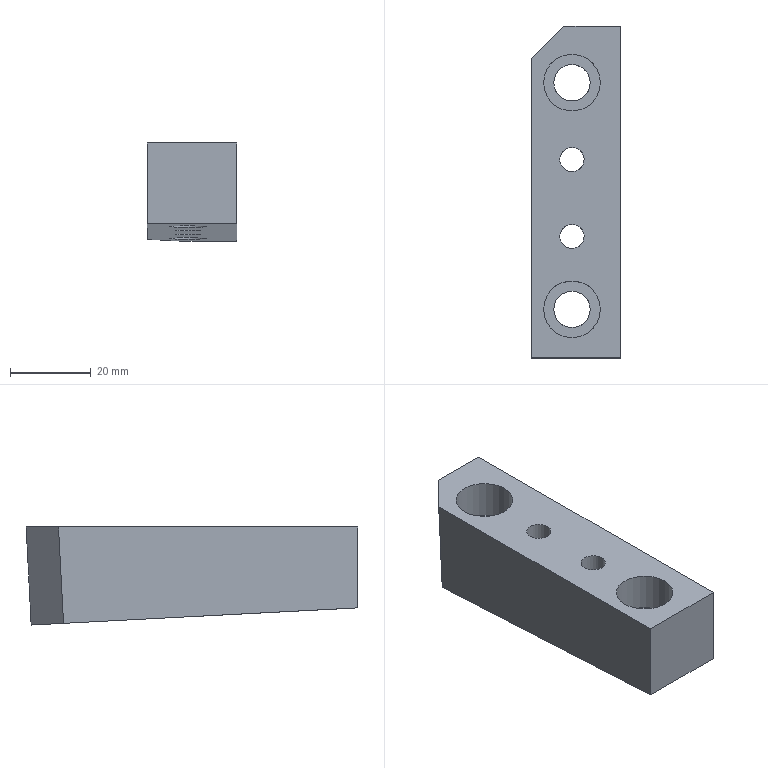Part | STEP file | P011002S001-004 | 1 solid | 15 faces | box 22 x 82 x 24.22 mm | volume 33052 mm3 | plane 9 | cylinder 6 | commonest cylinder face diameters 6 x2 9 x2 14 x2
STEP:
#1=CARTESIAN_POINT('',(0.,0.,0.));
#2=DIRECTION('',(0.,0.,1.));
#3=DIRECTION('',(1.,0.,0.));
#4=AXIS2_PLACEMENT_3D('',#1,#2,#3);
#5=CARTESIAN_POINT('',(-69.5,280.731,-5.22));
#6=VERTEX_POINT('',#5);
#7=CARTESIAN_POINT('',(-55.5,280.731,-5.22));
#8=VERTEX_POINT('',#7);
#9=CARTESIAN_POINT('',(-55.5,280.731,-5.22));
#10=DIRECTION('',(1.,0.,0.));
#11=VECTOR('',#10,1.);
#12=LINE('',#9,#11);
#13=CARTESIAN_POINT('',(-55.5,257.583,-4.007));
#14=DIRECTION('',(0.,-0.05234,-0.9986));
#15=DIRECTION('',(0.,-0.9986,0.05234));
#16=AXIS2_PLACEMENT_3D('',#13,#14,#15);
#17=PLANE('',#16);
#18=CARTESIAN_POINT('',(-23.18,0.));
#19=DIRECTION('',(0.,-1.));
#20=VECTOR('',#19,1.);
#21=LINE('',#18,#20);
#22=(GEOMETRIC_REPRESENTATION_CONTEXT(2)PARAMETRIC_REPRESENTATION_CONTEXT()REPRESENTATION_CONTEXT('',''));
#23=DEFINITIONAL_REPRESENTATION('',(#21),#22);
#24=PCURVE('',#17,#23);
#25=CARTESIAN_POINT('',(76.5,282.,19.));
#26=DIRECTION('',(0.,0.9986,-0.05234));
#27=DIRECTION('',(0.,0.05234,0.9986));
#28=AXIS2_PLACEMENT_3D('',#25,#26,#27);
#29=PLANE('',#28);
#30=CARTESIAN_POINT('',(-24.253,-132.));
#31=DIRECTION('',(0.,1.));
#32=VECTOR('',#31,1.);
#33=LINE('',#30,#32);
#34=(GEOMETRIC_REPRESENTATION_CONTEXT(2)PARAMETRIC_REPRESENTATION_CONTEXT()REPRESENTATION_CONTEXT('',''));
#35=DEFINITIONAL_REPRESENTATION('',(#33),#34);
#36=PCURVE('',#29,#35);
#37=SURFACE_CURVE('',#12,(#24,#36),.PCURVE_S1.);
#38=EDGE_CURVE('',#6,#8,#37,.T.);
#39=ORIENTED_EDGE('',*,*,#38,.T.);
#40=CARTESIAN_POINT('',(-55.5,200.,-0.989));
#41=VERTEX_POINT('',#40);
#42=CARTESIAN_POINT('',(-55.5,257.583,-4.007));
#43=DIRECTION('',(0.,-0.9986,0.05234));
#44=VECTOR('',#43,1.);
#45=LINE('',#42,#44);
#46=CARTESIAN_POINT('',(0.,0.));
#47=DIRECTION('',(1.,0.));
#48=VECTOR('',#47,1.);
#49=LINE('',#46,#48);
#50=(GEOMETRIC_REPRESENTATION_CONTEXT(2)PARAMETRIC_REPRESENTATION_CONTEXT()REPRESENTATION_CONTEXT('',''));
#51=DEFINITIONAL_REPRESENTATION('',(#49),#50);
#52=PCURVE('',#17,#51);
#53=CARTESIAN_POINT('',(-55.5,257.583,-4.007));
#54=DIRECTION('',(1.,0.,0.));
#55=DIRECTION('',(0.,0.,1.));
#56=AXIS2_PLACEMENT_3D('',#53,#54,#55);
#57=PLANE('',#56);
#58=CARTESIAN_POINT('',(0.,0.));
#59=DIRECTION('',(0.05234,0.9986));
#60=VECTOR('',#59,1.);
#61=LINE('',#58,#60);
#62=(GEOMETRIC_REPRESENTATION_CONTEXT(2)PARAMETRIC_REPRESENTATION_CONTEXT()REPRESENTATION_CONTEXT('',''));
#63=DEFINITIONAL_REPRESENTATION('',(#61),#62);
#64=PCURVE('',#57,#63);
#65=SURFACE_CURVE('',#45,(#52,#64),.PCURVE_S1.);
#66=EDGE_CURVE('',#8,#41,#65,.T.);
#67=ORIENTED_EDGE('',*,*,#66,.T.);
#68=CARTESIAN_POINT('',(-77.5,200.,-0.989));
#69=VERTEX_POINT('',#68);
#70=CARTESIAN_POINT('',(165.,200.,-0.989));
#71=DIRECTION('',(-1.,0.,0.));
#72=VECTOR('',#71,1.);
#73=LINE('',#70,#72);
#74=CARTESIAN_POINT('',(57.662,-220.5));
#75=DIRECTION('',(0.,1.));
#76=VECTOR('',#75,1.);
#77=LINE('',#74,#76);
#78=(GEOMETRIC_REPRESENTATION_CONTEXT(2)PARAMETRIC_REPRESENTATION_CONTEXT()REPRESENTATION_CONTEXT('',''));
#79=DEFINITIONAL_REPRESENTATION('',(#77),#78);
#80=PCURVE('',#17,#79);
#81=CARTESIAN_POINT('',(165.,200.,-50.));
#82=DIRECTION('',(0.,-1.,0.));
#83=DIRECTION('',(0.,0.,-1.));
#84=AXIS2_PLACEMENT_3D('',#81,#82,#83);
#85=PLANE('',#84);
#86=CARTESIAN_POINT('',(-49.011,0.));
#87=DIRECTION('',(0.,-1.));
#88=VECTOR('',#87,1.);
#89=LINE('',#86,#88);
#90=(GEOMETRIC_REPRESENTATION_CONTEXT(2)PARAMETRIC_REPRESENTATION_CONTEXT()REPRESENTATION_CONTEXT('',''));
#91=DEFINITIONAL_REPRESENTATION('',(#89),#90);
#92=PCURVE('',#85,#91);
#93=SURFACE_CURVE('',#73,(#80,#92),.PCURVE_S1.);
#94=EDGE_CURVE('',#41,#69,#93,.T.);
#95=ORIENTED_EDGE('',*,*,#94,.T.);
#96=CARTESIAN_POINT('',(-77.5,272.742,-4.801));
#97=VERTEX_POINT('',#96);
#98=CARTESIAN_POINT('',(-77.5,257.583,-4.007));
#99=DIRECTION('',(0.,-0.9986,0.05234));
#100=VECTOR('',#99,1.);
#101=LINE('',#98,#100);
#102=CARTESIAN_POINT('',(0.,22.));
#103=DIRECTION('',(1.,0.));
#104=VECTOR('',#103,1.);
#105=LINE('',#102,#104);
#106=(GEOMETRIC_REPRESENTATION_CONTEXT(2)PARAMETRIC_REPRESENTATION_CONTEXT()REPRESENTATION_CONTEXT('',''));
#107=DEFINITIONAL_REPRESENTATION('',(#105),#106);
#108=PCURVE('',#17,#107);
#109=CARTESIAN_POINT('',(-77.5,257.583,-4.007));
#110=DIRECTION('',(1.,0.,0.));
#111=DIRECTION('',(0.,0.,1.));
#112=AXIS2_PLACEMENT_3D('',#109,#110,#111);
#113=PLANE('',#112);
#114=CARTESIAN_POINT('',(0.,0.));
#115=DIRECTION('',(0.05234,0.9986));
#116=VECTOR('',#115,1.);
#117=LINE('',#114,#116);
#118=(GEOMETRIC_REPRESENTATION_CONTEXT(2)PARAMETRIC_REPRESENTATION_CONTEXT()REPRESENTATION_CONTEXT('',''));
#119=DEFINITIONAL_REPRESENTATION('',(#117),#118);
#120=PCURVE('',#113,#119);
#121=SURFACE_CURVE('',#101,(#108,#120),.PCURVE_S1.);
#122=EDGE_CURVE('',#97,#69,#121,.T.);
#123=ORIENTED_EDGE('',*,*,#122,.F.);
#124=CARTESIAN_POINT('',(-74.09,276.147,-4.98));
#125=DIRECTION('',(-0.7071,-0.7061,0.03701));
#126=VECTOR('',#125,1.);
#127=LINE('',#124,#126);
#128=CARTESIAN_POINT('',(-18.59,18.59));
#129=DIRECTION('',(0.7071,0.7071));
#130=VECTOR('',#129,1.);
#131=LINE('',#128,#130);
#132=(GEOMETRIC_REPRESENTATION_CONTEXT(2)PARAMETRIC_REPRESENTATION_CONTEXT()REPRESENTATION_CONTEXT('',''));
#133=DEFINITIONAL_REPRESENTATION('',(#131),#132);
#134=PCURVE('',#17,#133);
#135=CARTESIAN_POINT('',(-77.5,272.742,-4.801));
#136=DIRECTION('',(-0.7071,0.7061,-0.03701));
#137=DIRECTION('',(0.7066,0.7076,0.));
#138=AXIS2_PLACEMENT_3D('',#135,#136,#137);
#139=PLANE('',#138);
#140=CARTESIAN_POINT('',(4.819,0.1786));
#141=DIRECTION('',(-0.9993,-0.03703));
#142=VECTOR('',#141,1.);
#143=LINE('',#140,#142);
#144=(GEOMETRIC_REPRESENTATION_CONTEXT(2)PARAMETRIC_REPRESENTATION_CONTEXT()REPRESENTATION_CONTEXT('',''));
#145=DEFINITIONAL_REPRESENTATION('',(#143),#144);
#146=PCURVE('',#139,#145);
#147=SURFACE_CURVE('',#127,(#134,#146),.PCURVE_S1.);
#148=EDGE_CURVE('',#6,#97,#147,.T.);
#149=ORIENTED_EDGE('',*,*,#148,.F.);
#150=EDGE_LOOP('',(#39,#67,#95,#123,#149));
#151=FACE_BOUND('',#150,.T.);
#152=CARTESIAN_POINT('',(-67.5,272.5,-4.789));
#153=VERTEX_POINT('',#152);
#154=CARTESIAN_POINT('',(-63.,268.,-4.553));
#155=VERTEX_POINT('',#154);
#156=CARTESIAN_POINT('',(-67.5,268.,-4.553));
#157=DIRECTION('',(0.,-0.05234,-0.9986));
#158=DIRECTION('',(0.,0.9986,-0.05234));
#159=AXIS2_PLACEMENT_3D('',#156,#157,#158);
#160=ELLIPSE('',#159,4.506,4.5);
#161=CARTESIAN_POINT('',(-10.431,12.));
#162=DIRECTION('',(-1.,0.));
#163=AXIS2_PLACEMENT_2D('',#161,#162);
#164=ELLIPSE('',#163,4.506,4.5);
#165=(GEOMETRIC_REPRESENTATION_CONTEXT(2)PARAMETRIC_REPRESENTATION_CONTEXT()REPRESENTATION_CONTEXT('',''));
#166=DEFINITIONAL_REPRESENTATION('',(#164),#165);
#167=PCURVE('',#17,#166);
#168=CARTESIAN_POINT('',(-67.5,268.,19.));
#169=DIRECTION('',(0.,0.,-1.));
#170=DIRECTION('',(1.,0.,0.));
#171=AXIS2_PLACEMENT_3D('',#168,#169,#170);
#172=CYLINDRICAL_SURFACE('',#171,4.5);
#173=CARTESIAN_POINT('',(4.712,23.789));
#174=CARTESIAN_POINT('',(4.808,23.789));
#175=CARTESIAN_POINT('',(4.998,23.782));
#176=CARTESIAN_POINT('',(5.284,23.754));
#177=CARTESIAN_POINT('',(5.569,23.709));
#178=CARTESIAN_POINT('',(5.855,23.652));
#179=CARTESIAN_POINT('',(6.14,23.587));
#180=CARTESIAN_POINT('',(6.426,23.519));
#181=CARTESIAN_POINT('',(6.712,23.453));
#182=CARTESIAN_POINT('',(6.997,23.396));
#183=CARTESIAN_POINT('',(7.283,23.352));
#184=CARTESIAN_POINT('',(7.568,23.323));
#185=CARTESIAN_POINT('',(7.854,23.314));
#186=CARTESIAN_POINT('',(8.14,23.323));
#187=CARTESIAN_POINT('',(8.425,23.352));
#188=CARTESIAN_POINT('',(8.711,23.396));
#189=CARTESIAN_POINT('',(8.996,23.453));
#190=CARTESIAN_POINT('',(9.282,23.519));
#191=CARTESIAN_POINT('',(9.568,23.587));
#192=CARTESIAN_POINT('',(9.853,23.652));
#193=CARTESIAN_POINT('',(10.139,23.709));
#194=CARTESIAN_POINT('',(10.424,23.754));
#195=CARTESIAN_POINT('',(10.71,23.782));
#196=CARTESIAN_POINT('',(10.9,23.789));
#197=CARTESIAN_POINT('',(10.996,23.789));
#198=B_SPLINE_CURVE_WITH_KNOTS('',3,(#173,#174,#175,#176,#177,#178,#179,#180,#181,#182,#183,#184,#185,#186,#187,#188,#189,#190,#191,#192,#193,#194,#195,#196,#197),.UNSPECIFIED.,.F.,.F.,(4,1,1,1,1,1,1,1,1,1,1,1,1,1,1,1,1,1,1,1,1,1,4),(0.,0.2856,0.5712,0.8568,1.142,1.428,1.714,1.999,2.285,2.57,2.856,3.142,3.427,3.713,3.998,4.284,4.57,4.855,5.141,5.426,5.712,5.998,6.283),.QUASI_UNIFORM_KNOTS.);
#199=(GEOMETRIC_REPRESENTATION_CONTEXT(2)PARAMETRIC_REPRESENTATION_CONTEXT()REPRESENTATION_CONTEXT('',''));
#200=DEFINITIONAL_REPRESENTATION('',(#198),#199);
#201=PCURVE('',#172,#200);
#202=SURFACE_CURVE('',#160,(#167,#201),.PCURVE_S1.);
#203=EDGE_CURVE('',#153,#155,#202,.T.);
#204=ORIENTED_EDGE('',*,*,#203,.F.);
#205=CARTESIAN_POINT('',(-67.5,268.,-4.553));
#206=DIRECTION('',(0.,-0.05234,-0.9986));
#207=DIRECTION('',(0.,0.9986,-0.05234));
#208=AXIS2_PLACEMENT_3D('',#205,#206,#207);
#209=ELLIPSE('',#208,4.506,4.5);
#210=CARTESIAN_POINT('',(-10.431,12.));
#211=DIRECTION('',(-1.,0.));
#212=AXIS2_PLACEMENT_2D('',#210,#211);
#213=ELLIPSE('',#212,4.506,4.5);
#214=(GEOMETRIC_REPRESENTATION_CONTEXT(2)PARAMETRIC_REPRESENTATION_CONTEXT()REPRESENTATION_CONTEXT('',''));
#215=DEFINITIONAL_REPRESENTATION('',(#213),#214);
#216=PCURVE('',#17,#215);
#217=CARTESIAN_POINT('',(-1.571,23.789));
#218=CARTESIAN_POINT('',(-1.476,23.789));
#219=CARTESIAN_POINT('',(-1.285,23.782));
#220=CARTESIAN_POINT('',(-0.9996,23.754));
#221=CARTESIAN_POINT('',(-0.714,23.709));
#222=CARTESIAN_POINT('',(-0.4284,23.652));
#223=CARTESIAN_POINT('',(-0.1428,23.587));
#224=CARTESIAN_POINT('',(0.1428,23.519));
#225=CARTESIAN_POINT('',(0.4284,23.453));
#226=CARTESIAN_POINT('',(0.714,23.396));
#227=CARTESIAN_POINT('',(0.9996,23.352));
#228=CARTESIAN_POINT('',(1.285,23.323));
#229=CARTESIAN_POINT('',(1.571,23.314));
#230=CARTESIAN_POINT('',(1.856,23.323));
#231=CARTESIAN_POINT('',(2.142,23.352));
#232=CARTESIAN_POINT('',(2.428,23.396));
#233=CARTESIAN_POINT('',(2.713,23.453));
#234=CARTESIAN_POINT('',(2.999,23.519));
#235=CARTESIAN_POINT('',(3.284,23.587));
#236=CARTESIAN_POINT('',(3.57,23.652));
#237=CARTESIAN_POINT('',(3.856,23.709));
#238=CARTESIAN_POINT('',(4.141,23.754));
#239=CARTESIAN_POINT('',(4.427,23.782));
#240=CARTESIAN_POINT('',(4.617,23.789));
#241=CARTESIAN_POINT('',(4.712,23.789));
#242=B_SPLINE_CURVE_WITH_KNOTS('',3,(#217,#218,#219,#220,#221,#222,#223,#224,#225,#226,#227,#228,#229,#230,#231,#232,#233,#234,#235,#236,#237,#238,#239,#240,#241),.UNSPECIFIED.,.F.,.F.,(4,1,1,1,1,1,1,1,1,1,1,1,1,1,1,1,1,1,1,1,1,1,4),(0.,0.2856,0.5712,0.8568,1.142,1.428,1.714,1.999,2.285,2.57,2.856,3.142,3.427,3.713,3.998,4.284,4.57,4.855,5.141,5.426,5.712,5.998,6.283),.QUASI_UNIFORM_KNOTS.);
#243=(GEOMETRIC_REPRESENTATION_CONTEXT(2)PARAMETRIC_REPRESENTATION_CONTEXT()REPRESENTATION_CONTEXT('',''));
#244=DEFINITIONAL_REPRESENTATION('',(#242),#243);
#245=PCURVE('',#172,#244);
#246=SURFACE_CURVE('',#209,(#216,#245),.PCURVE_S1.);
#247=EDGE_CURVE('',#155,#153,#246,.T.);
#248=ORIENTED_EDGE('',*,*,#247,.F.);
#249=EDGE_LOOP('',(#204,#248));
#250=FACE_BOUND('',#249,.T.);
#251=CARTESIAN_POINT('',(-67.5,252.,-3.714));
#252=VERTEX_POINT('',#251);
#253=CARTESIAN_POINT('',(-67.5,249.,-3.557));
#254=DIRECTION('',(0.,-0.05234,-0.9986));
#255=DIRECTION('',(0.,0.9986,-0.05234));
#256=AXIS2_PLACEMENT_3D('',#253,#254,#255);
#257=ELLIPSE('',#256,3.004,3.);
#258=CARTESIAN_POINT('',(8.595,12.));
#259=DIRECTION('',(-1.,0.));
#260=AXIS2_PLACEMENT_2D('',#258,#259);
#261=ELLIPSE('',#260,3.004,3.);
#262=(GEOMETRIC_REPRESENTATION_CONTEXT(2)PARAMETRIC_REPRESENTATION_CONTEXT()REPRESENTATION_CONTEXT('',''));
#263=DEFINITIONAL_REPRESENTATION('',(#261),#262);
#264=PCURVE('',#17,#263);
#265=CARTESIAN_POINT('',(-67.5,249.,19.));
#266=DIRECTION('',(0.,0.,-1.));
#267=DIRECTION('',(1.,0.,0.));
#268=AXIS2_PLACEMENT_3D('',#265,#266,#267);
#269=CYLINDRICAL_SURFACE('',#268,3.);
#270=CARTESIAN_POINT('',(4.712,22.714));
#271=CARTESIAN_POINT('',(4.808,22.714));
#272=CARTESIAN_POINT('',(4.998,22.71));
#273=CARTESIAN_POINT('',(5.284,22.691));
#274=CARTESIAN_POINT('',(5.569,22.661));
#275=CARTESIAN_POINT('',(5.855,22.623));
#276=CARTESIAN_POINT('',(6.14,22.58));
#277=CARTESIAN_POINT('',(6.426,22.534));
#278=CARTESIAN_POINT('',(6.712,22.491));
#279=CARTESIAN_POINT('',(6.997,22.453));
#280=CARTESIAN_POINT('',(7.283,22.423));
#281=CARTESIAN_POINT('',(7.568,22.404));
#282=CARTESIAN_POINT('',(7.854,22.398));
#283=CARTESIAN_POINT('',(8.14,22.404));
#284=CARTESIAN_POINT('',(8.425,22.423));
#285=CARTESIAN_POINT('',(8.711,22.453));
#286=CARTESIAN_POINT('',(8.996,22.491));
#287=CARTESIAN_POINT('',(9.282,22.534));
#288=CARTESIAN_POINT('',(9.568,22.58));
#289=CARTESIAN_POINT('',(9.853,22.623));
#290=CARTESIAN_POINT('',(10.139,22.661));
#291=CARTESIAN_POINT('',(10.424,22.691));
#292=CARTESIAN_POINT('',(10.71,22.71));
#293=CARTESIAN_POINT('',(10.9,22.714));
#294=CARTESIAN_POINT('',(10.996,22.714));
#295=B_SPLINE_CURVE_WITH_KNOTS('',3,(#270,#271,#272,#273,#274,#275,#276,#277,#278,#279,#280,#281,#282,#283,#284,#285,#286,#287,#288,#289,#290,#291,#292,#293,#294),.UNSPECIFIED.,.F.,.F.,(4,1,1,1,1,1,1,1,1,1,1,1,1,1,1,1,1,1,1,1,1,1,4),(0.,0.2856,0.5712,0.8568,1.142,1.428,1.714,1.999,2.285,2.57,2.856,3.142,3.427,3.713,3.998,4.284,4.57,4.855,5.141,5.426,5.712,5.998,6.283),.QUASI_UNIFORM_KNOTS.);
#296=(GEOMETRIC_REPRESENTATION_CONTEXT(2)PARAMETRIC_REPRESENTATION_CONTEXT()REPRESENTATION_CONTEXT('',''));
#297=DEFINITIONAL_REPRESENTATION('',(#295),#296);
#298=PCURVE('',#269,#297);
#299=SURFACE_CURVE('',#257,(#264,#298),.PCURVE_S1.);
#300=EDGE_CURVE('',#252,#252,#299,.T.);
#301=ORIENTED_EDGE('',*,*,#300,.F.);
#302=EDGE_LOOP('',(#301));
#303=FACE_BOUND('',#302,.T.);
#304=CARTESIAN_POINT('',(-67.5,233.,-2.718));
#305=VERTEX_POINT('',#304);
#306=CARTESIAN_POINT('',(-67.5,230.,-2.561));
#307=DIRECTION('',(0.,-0.05234,-0.9986));
#308=DIRECTION('',(0.,0.9986,-0.05234));
#309=AXIS2_PLACEMENT_3D('',#306,#307,#308);
#310=ELLIPSE('',#309,3.004,3.);
#311=CARTESIAN_POINT('',(27.621,12.));
#312=DIRECTION('',(-1.,0.));
#313=AXIS2_PLACEMENT_2D('',#311,#312);
#314=ELLIPSE('',#313,3.004,3.);
#315=(GEOMETRIC_REPRESENTATION_CONTEXT(2)PARAMETRIC_REPRESENTATION_CONTEXT()REPRESENTATION_CONTEXT('',''));
#316=DEFINITIONAL_REPRESENTATION('',(#314),#315);
#317=PCURVE('',#17,#316);
#318=CARTESIAN_POINT('',(-67.5,230.,19.));
#319=DIRECTION('',(0.,0.,-1.));
#320=DIRECTION('',(1.,0.,0.));
#321=AXIS2_PLACEMENT_3D('',#318,#319,#320);
#322=CYLINDRICAL_SURFACE('',#321,3.);
#323=CARTESIAN_POINT('',(4.712,21.718));
#324=CARTESIAN_POINT('',(4.808,21.719));
#325=CARTESIAN_POINT('',(4.998,21.714));
#326=CARTESIAN_POINT('',(5.284,21.695));
#327=CARTESIAN_POINT('',(5.569,21.666));
#328=CARTESIAN_POINT('',(5.855,21.627));
#329=CARTESIAN_POINT('',(6.14,21.584));
#330=CARTESIAN_POINT('',(6.426,21.539));
#331=CARTESIAN_POINT('',(6.712,21.495));
#332=CARTESIAN_POINT('',(6.997,21.457));
#333=CARTESIAN_POINT('',(7.283,21.427));
#334=CARTESIAN_POINT('',(7.568,21.408));
#335=CARTESIAN_POINT('',(7.854,21.402));
#336=CARTESIAN_POINT('',(8.14,21.408));
#337=CARTESIAN_POINT('',(8.425,21.427));
#338=CARTESIAN_POINT('',(8.711,21.457));
#339=CARTESIAN_POINT('',(8.996,21.495));
#340=CARTESIAN_POINT('',(9.282,21.539));
#341=CARTESIAN_POINT('',(9.568,21.584));
#342=CARTESIAN_POINT('',(9.853,21.627));
#343=CARTESIAN_POINT('',(10.139,21.666));
#344=CARTESIAN_POINT('',(10.424,21.695));
#345=CARTESIAN_POINT('',(10.71,21.714));
#346=CARTESIAN_POINT('',(10.9,21.719));
#347=CARTESIAN_POINT('',(10.996,21.718));
#348=B_SPLINE_CURVE_WITH_KNOTS('',3,(#323,#324,#325,#326,#327,#328,#329,#330,#331,#332,#333,#334,#335,#336,#337,#338,#339,#340,#341,#342,#343,#344,#345,#346,#347),.UNSPECIFIED.,.F.,.F.,(4,1,1,1,1,1,1,1,1,1,1,1,1,1,1,1,1,1,1,1,1,1,4),(0.,0.2856,0.5712,0.8568,1.142,1.428,1.714,1.999,2.285,2.57,2.856,3.142,3.427,3.713,3.998,4.284,4.57,4.855,5.141,5.426,5.712,5.998,6.283),.QUASI_UNIFORM_KNOTS.);
#349=(GEOMETRIC_REPRESENTATION_CONTEXT(2)PARAMETRIC_REPRESENTATION_CONTEXT()REPRESENTATION_CONTEXT('',''));
#350=DEFINITIONAL_REPRESENTATION('',(#348),#349);
#351=PCURVE('',#322,#350);
#352=SURFACE_CURVE('',#310,(#317,#351),.PCURVE_S1.);
#353=EDGE_CURVE('',#305,#305,#352,.T.);
#354=ORIENTED_EDGE('',*,*,#353,.F.);
#355=EDGE_LOOP('',(#354));
#356=FACE_BOUND('',#355,.T.);
#357=CARTESIAN_POINT('',(-67.5,216.5,-1.854));
#358=VERTEX_POINT('',#357);
#359=CARTESIAN_POINT('',(-63.,212.,-1.618));
#360=VERTEX_POINT('',#359);
#361=CARTESIAN_POINT('',(-67.5,212.,-1.618));
#362=DIRECTION('',(0.,-0.05234,-0.9986));
#363=DIRECTION('',(0.,0.9986,-0.05234));
#364=AXIS2_PLACEMENT_3D('',#361,#362,#363);
#365=ELLIPSE('',#364,4.506,4.5);
#366=CARTESIAN_POINT('',(45.645,12.));
#367=DIRECTION('',(-1.,0.));
#368=AXIS2_PLACEMENT_2D('',#366,#367);
#369=ELLIPSE('',#368,4.506,4.5);
#370=(GEOMETRIC_REPRESENTATION_CONTEXT(2)PARAMETRIC_REPRESENTATION_CONTEXT()REPRESENTATION_CONTEXT('',''));
#371=DEFINITIONAL_REPRESENTATION('',(#369),#370);
#372=PCURVE('',#17,#371);
#373=CARTESIAN_POINT('',(-67.5,212.,19.));
#374=DIRECTION('',(0.,0.,-1.));
#375=DIRECTION('',(1.,0.,0.));
#376=AXIS2_PLACEMENT_3D('',#373,#374,#375);
#377=CYLINDRICAL_SURFACE('',#376,4.5);
#378=CARTESIAN_POINT('',(4.712,20.854));
#379=CARTESIAN_POINT('',(4.808,20.854));
#380=CARTESIAN_POINT('',(4.998,20.847));
#381=CARTESIAN_POINT('',(5.284,20.819));
#382=CARTESIAN_POINT('',(5.569,20.774));
#383=CARTESIAN_POINT('',(5.855,20.717));
#384=CARTESIAN_POINT('',(6.14,20.652));
#385=CARTESIAN_POINT('',(6.426,20.584));
#386=CARTESIAN_POINT('',(6.712,20.519));
#387=CARTESIAN_POINT('',(6.997,20.461));
#388=CARTESIAN_POINT('',(7.283,20.417));
#389=CARTESIAN_POINT('',(7.568,20.389));
#390=CARTESIAN_POINT('',(7.854,20.379));
#391=CARTESIAN_POINT('',(8.14,20.389));
#392=CARTESIAN_POINT('',(8.425,20.417));
#393=CARTESIAN_POINT('',(8.711,20.461));
#394=CARTESIAN_POINT('',(8.996,20.519));
#395=CARTESIAN_POINT('',(9.282,20.584));
#396=CARTESIAN_POINT('',(9.568,20.652));
#397=CARTESIAN_POINT('',(9.853,20.717));
#398=CARTESIAN_POINT('',(10.139,20.774));
#399=CARTESIAN_POINT('',(10.424,20.819));
#400=CARTESIAN_POINT('',(10.71,20.847));
#401=CARTESIAN_POINT('',(10.9,20.854));
#402=CARTESIAN_POINT('',(10.996,20.854));
#403=B_SPLINE_CURVE_WITH_KNOTS('',3,(#378,#379,#380,#381,#382,#383,#384,#385,#386,#387,#388,#389,#390,#391,#392,#393,#394,#395,#396,#397,#398,#399,#400,#401,#402),.UNSPECIFIED.,.F.,.F.,(4,1,1,1,1,1,1,1,1,1,1,1,1,1,1,1,1,1,1,1,1,1,4),(0.,0.2856,0.5712,0.8568,1.142,1.428,1.714,1.999,2.285,2.57,2.856,3.142,3.427,3.713,3.998,4.284,4.57,4.855,5.141,5.426,5.712,5.998,6.283),.QUASI_UNIFORM_KNOTS.);
#404=(GEOMETRIC_REPRESENTATION_CONTEXT(2)PARAMETRIC_REPRESENTATION_CONTEXT()REPRESENTATION_CONTEXT('',''));
#405=DEFINITIONAL_REPRESENTATION('',(#403),#404);
#406=PCURVE('',#377,#405);
#407=SURFACE_CURVE('',#365,(#372,#406),.PCURVE_S1.);
#408=EDGE_CURVE('',#358,#360,#407,.T.);
#409=ORIENTED_EDGE('',*,*,#408,.F.);
#410=CARTESIAN_POINT('',(-67.5,212.,-1.618));
#411=DIRECTION('',(0.,-0.05234,-0.9986));
#412=DIRECTION('',(0.,0.9986,-0.05234));
#413=AXIS2_PLACEMENT_3D('',#410,#411,#412);
#414=ELLIPSE('',#413,4.506,4.5);
#415=CARTESIAN_POINT('',(45.645,12.));
#416=DIRECTION('',(-1.,0.));
#417=AXIS2_PLACEMENT_2D('',#415,#416);
#418=ELLIPSE('',#417,4.506,4.5);
#419=(GEOMETRIC_REPRESENTATION_CONTEXT(2)PARAMETRIC_REPRESENTATION_CONTEXT()REPRESENTATION_CONTEXT('',''));
#420=DEFINITIONAL_REPRESENTATION('',(#418),#419);
#421=PCURVE('',#17,#420);
#422=CARTESIAN_POINT('',(-1.571,20.854));
#423=CARTESIAN_POINT('',(-1.476,20.854));
#424=CARTESIAN_POINT('',(-1.285,20.847));
#425=CARTESIAN_POINT('',(-0.9996,20.819));
#426=CARTESIAN_POINT('',(-0.714,20.774));
#427=CARTESIAN_POINT('',(-0.4284,20.717));
#428=CARTESIAN_POINT('',(-0.1428,20.652));
#429=CARTESIAN_POINT('',(0.1428,20.584));
#430=CARTESIAN_POINT('',(0.4284,20.519));
#431=CARTESIAN_POINT('',(0.714,20.461));
#432=CARTESIAN_POINT('',(0.9996,20.417));
#433=CARTESIAN_POINT('',(1.285,20.389));
#434=CARTESIAN_POINT('',(1.571,20.379));
#435=CARTESIAN_POINT('',(1.856,20.389));
#436=CARTESIAN_POINT('',(2.142,20.417));
#437=CARTESIAN_POINT('',(2.428,20.461));
#438=CARTESIAN_POINT('',(2.713,20.519));
#439=CARTESIAN_POINT('',(2.999,20.584));
#440=CARTESIAN_POINT('',(3.284,20.652));
#441=CARTESIAN_POINT('',(3.57,20.717));
#442=CARTESIAN_POINT('',(3.856,20.774));
#443=CARTESIAN_POINT('',(4.141,20.819));
#444=CARTESIAN_POINT('',(4.427,20.847));
#445=CARTESIAN_POINT('',(4.617,20.854));
#446=CARTESIAN_POINT('',(4.712,20.854));
#447=B_SPLINE_CURVE_WITH_KNOTS('',3,(#422,#423,#424,#425,#426,#427,#428,#429,#430,#431,#432,#433,#434,#435,#436,#437,#438,#439,#440,#441,#442,#443,#444,#445,#446),.UNSPECIFIED.,.F.,.F.,(4,1,1,1,1,1,1,1,1,1,1,1,1,1,1,1,1,1,1,1,1,1,4),(0.,0.2856,0.5712,0.8568,1.142,1.428,1.714,1.999,2.285,2.57,2.856,3.142,3.427,3.713,3.998,4.284,4.57,4.855,5.141,5.426,5.712,5.998,6.283),.QUASI_UNIFORM_KNOTS.);
#448=(GEOMETRIC_REPRESENTATION_CONTEXT(2)PARAMETRIC_REPRESENTATION_CONTEXT()REPRESENTATION_CONTEXT('',''));
#449=DEFINITIONAL_REPRESENTATION('',(#447),#448);
#450=PCURVE('',#377,#449);
#451=SURFACE_CURVE('',#414,(#421,#450),.PCURVE_S1.);
#452=EDGE_CURVE('',#360,#358,#451,.T.);
#453=ORIENTED_EDGE('',*,*,#452,.F.);
#454=EDGE_LOOP('',(#409,#453));
#455=FACE_BOUND('',#454,.T.);
#456=ADVANCED_FACE('',(#151,#250,#303,#356,#455),#17,.T.);
#457=CARTESIAN_POINT('',(-77.5,273.989,19.));
#458=VERTEX_POINT('',#457);
#459=CARTESIAN_POINT('',(-77.5,200.,19.));
#460=VERTEX_POINT('',#459);
#461=CARTESIAN_POINT('',(-77.5,-325.,19.));
#462=DIRECTION('',(0.,-1.,0.));
#463=VECTOR('',#462,1.);
#464=LINE('',#461,#463);
#465=CARTESIAN_POINT('',(-275.,-325.,19.));
#466=DIRECTION('',(0.,0.,1.));
#467=DIRECTION('',(-1.,0.,0.));
#468=AXIS2_PLACEMENT_3D('',#465,#466,#467);
#469=PLANE('',#468);
#470=CARTESIAN_POINT('',(-197.5,0.));
#471=DIRECTION('',(0.,1.));
#472=VECTOR('',#471,1.);
#473=LINE('',#470,#472);
#474=(GEOMETRIC_REPRESENTATION_CONTEXT(2)PARAMETRIC_REPRESENTATION_CONTEXT()REPRESENTATION_CONTEXT('',''));
#475=DEFINITIONAL_REPRESENTATION('',(#473),#474);
#476=PCURVE('',#469,#475);
#477=CARTESIAN_POINT('',(23.007,582.583));
#478=DIRECTION('',(0.,1.));
#479=VECTOR('',#478,1.);
#480=LINE('',#477,#479);
#481=(GEOMETRIC_REPRESENTATION_CONTEXT(2)PARAMETRIC_REPRESENTATION_CONTEXT()REPRESENTATION_CONTEXT('',''));
#482=DEFINITIONAL_REPRESENTATION('',(#480),#481);
#483=PCURVE('',#113,#482);
#484=SURFACE_CURVE('',#464,(#476,#483),.PCURVE_S1.);
#485=EDGE_CURVE('',#458,#460,#484,.T.);
#486=ORIENTED_EDGE('',*,*,#485,.T.);
#487=CARTESIAN_POINT('',(-55.5,200.,19.));
#488=VERTEX_POINT('',#487);
#489=CARTESIAN_POINT('',(-275.,200.,19.));
#490=DIRECTION('',(-1.,0.,0.));
#491=VECTOR('',#490,1.);
#492=LINE('',#489,#491);
#493=CARTESIAN_POINT('',(0.,-525.));
#494=DIRECTION('',(1.,0.));
#495=VECTOR('',#494,1.);
#496=LINE('',#493,#495);
#497=(GEOMETRIC_REPRESENTATION_CONTEXT(2)PARAMETRIC_REPRESENTATION_CONTEXT()REPRESENTATION_CONTEXT('',''));
#498=DEFINITIONAL_REPRESENTATION('',(#496),#497);
#499=PCURVE('',#469,#498);
#500=CARTESIAN_POINT('',(-69.,-440.));
#501=DIRECTION('',(0.,-1.));
#502=VECTOR('',#501,1.);
#503=LINE('',#500,#502);
#504=(GEOMETRIC_REPRESENTATION_CONTEXT(2)PARAMETRIC_REPRESENTATION_CONTEXT()REPRESENTATION_CONTEXT('',''));
#505=DEFINITIONAL_REPRESENTATION('',(#503),#504);
#506=PCURVE('',#85,#505);
#507=SURFACE_CURVE('',#492,(#499,#506),.PCURVE_S1.);
#508=EDGE_CURVE('',#488,#460,#507,.T.);
#509=ORIENTED_EDGE('',*,*,#508,.F.);
#510=CARTESIAN_POINT('',(-55.5,282.,19.));
#511=VERTEX_POINT('',#510);
#512=CARTESIAN_POINT('',(-55.5,-325.,19.));
#513=DIRECTION('',(0.,-1.,0.));
#514=VECTOR('',#513,1.);
#515=LINE('',#512,#514);
#516=CARTESIAN_POINT('',(-219.5,0.));
#517=DIRECTION('',(0.,1.));
#518=VECTOR('',#517,1.);
#519=LINE('',#516,#518);
#520=(GEOMETRIC_REPRESENTATION_CONTEXT(2)PARAMETRIC_REPRESENTATION_CONTEXT()REPRESENTATION_CONTEXT('',''));
#521=DEFINITIONAL_REPRESENTATION('',(#519),#520);
#522=PCURVE('',#469,#521);
#523=CARTESIAN_POINT('',(23.007,582.583));
#524=DIRECTION('',(0.,1.));
#525=VECTOR('',#524,1.);
#526=LINE('',#523,#525);
#527=(GEOMETRIC_REPRESENTATION_CONTEXT(2)PARAMETRIC_REPRESENTATION_CONTEXT()REPRESENTATION_CONTEXT('',''));
#528=DEFINITIONAL_REPRESENTATION('',(#526),#527);
#529=PCURVE('',#57,#528);
#530=SURFACE_CURVE('',#515,(#522,#529),.PCURVE_S1.);
#531=EDGE_CURVE('',#511,#488,#530,.T.);
#532=ORIENTED_EDGE('',*,*,#531,.F.);
#533=CARTESIAN_POINT('',(-69.5,282.,19.));
#534=VERTEX_POINT('',#533);
#535=CARTESIAN_POINT('',(-275.,282.,19.));
#536=DIRECTION('',(-1.,0.,0.));
#537=VECTOR('',#536,1.);
#538=LINE('',#535,#537);
#539=CARTESIAN_POINT('',(0.,-607.));
#540=DIRECTION('',(1.,0.));
#541=VECTOR('',#540,1.);
#542=LINE('',#539,#541);
#543=(GEOMETRIC_REPRESENTATION_CONTEXT(2)PARAMETRIC_REPRESENTATION_CONTEXT()REPRESENTATION_CONTEXT('',''));
#544=DEFINITIONAL_REPRESENTATION('',(#542),#543);
#545=PCURVE('',#469,#544);
#546=CARTESIAN_POINT('',(0.,-351.5));
#547=DIRECTION('',(0.,-1.));
#548=VECTOR('',#547,1.);
#549=LINE('',#546,#548);
#550=(GEOMETRIC_REPRESENTATION_CONTEXT(2)PARAMETRIC_REPRESENTATION_CONTEXT()REPRESENTATION_CONTEXT('',''));
#551=DEFINITIONAL_REPRESENTATION('',(#549),#550);
#552=PCURVE('',#29,#551);
#553=SURFACE_CURVE('',#538,(#545,#552),.PCURVE_S1.);
#554=EDGE_CURVE('',#511,#534,#553,.T.);
#555=ORIENTED_EDGE('',*,*,#554,.T.);
#556=CARTESIAN_POINT('',(-475.609,-124.666,19.));
#557=DIRECTION('',(0.7066,0.7076,0.));
#558=VECTOR('',#557,1.);
#559=LINE('',#556,#558);
#560=CARTESIAN_POINT('',(200.609,-200.334));
#561=DIRECTION('',(-0.7066,-0.7076));
#562=VECTOR('',#561,1.);
#563=LINE('',#560,#562);
#564=(GEOMETRIC_REPRESENTATION_CONTEXT(2)PARAMETRIC_REPRESENTATION_CONTEXT()REPRESENTATION_CONTEXT('',''));
#565=DEFINITIONAL_REPRESENTATION('',(#563),#564);
#566=PCURVE('',#469,#565);
#567=CARTESIAN_POINT('',(-562.515,-23.818));
#568=DIRECTION('',(1.,0.));
#569=VECTOR('',#568,1.);
#570=LINE('',#567,#569);
#571=(GEOMETRIC_REPRESENTATION_CONTEXT(2)PARAMETRIC_REPRESENTATION_CONTEXT()REPRESENTATION_CONTEXT('',''));
#572=DEFINITIONAL_REPRESENTATION('',(#570),#571);
#573=PCURVE('',#139,#572);
#574=SURFACE_CURVE('',#559,(#566,#573),.PCURVE_S1.);
#575=EDGE_CURVE('',#458,#534,#574,.T.);
#576=ORIENTED_EDGE('',*,*,#575,.F.);
#577=EDGE_LOOP('',(#486,#509,#532,#555,#576));
#578=FACE_BOUND('',#577,.T.);
#579=CARTESIAN_POINT('',(-74.5,212.,19.));
#580=VERTEX_POINT('',#579);
#581=CARTESIAN_POINT('',(-67.5,212.,19.));
#582=DIRECTION('',(0.,0.,-1.));
#583=DIRECTION('',(-1.,0.,0.));
#584=AXIS2_PLACEMENT_3D('',#581,#582,#583);
#585=CIRCLE('',#584,7.);
#586=CARTESIAN_POINT('',(-200.5,-537.));
#587=CARTESIAN_POINT('',(-200.5,-549.124));
#588=CARTESIAN_POINT('',(-211.,-543.062));
#589=CARTESIAN_POINT('',(-221.5,-537.));
#590=CARTESIAN_POINT('',(-211.,-530.938));
#591=CARTESIAN_POINT('',(-200.5,-524.876));
#592=CARTESIAN_POINT('',(-200.5,-537.));
#593=(BOUNDED_CURVE()B_SPLINE_CURVE(2,(#586,#587,#588,#589,#590,#591,#592),.UNSPECIFIED.,.T.,.F.)B_SPLINE_CURVE_WITH_KNOTS((1,2,2,2,2,1),(-2.094,0.,2.094,4.189,6.283,8.378),.UNSPECIFIED.)CURVE()GEOMETRIC_REPRESENTATION_ITEM()RATIONAL_B_SPLINE_CURVE((1.,0.5,1.,0.5,1.,0.5,1.))REPRESENTATION_ITEM(''));
#594=(GEOMETRIC_REPRESENTATION_CONTEXT(2)PARAMETRIC_REPRESENTATION_CONTEXT()REPRESENTATION_CONTEXT('',''));
#595=DEFINITIONAL_REPRESENTATION('',(#593),#594);
#596=PCURVE('',#469,#595);
#597=CARTESIAN_POINT('',(-67.5,212.,19.));
#598=DIRECTION('',(0.,0.,-1.));
#599=DIRECTION('',(1.,0.,0.));
#600=AXIS2_PLACEMENT_3D('',#597,#598,#599);
#601=CYLINDRICAL_SURFACE('',#600,7.);
#602=CARTESIAN_POINT('',(3.142,0.));
#603=DIRECTION('',(1.,0.));
#604=VECTOR('',#603,1.);
#605=LINE('',#602,#604);
#606=(GEOMETRIC_REPRESENTATION_CONTEXT(2)PARAMETRIC_REPRESENTATION_CONTEXT()REPRESENTATION_CONTEXT('',''));
#607=DEFINITIONAL_REPRESENTATION('',(#605),#606);
#608=PCURVE('',#601,#607);
#609=SURFACE_CURVE('',#585,(#596,#608),.PCURVE_S1.);
#610=EDGE_CURVE('',#580,#580,#609,.T.);
#611=ORIENTED_EDGE('',*,*,#610,.T.);
#612=EDGE_LOOP('',(#611));
#613=FACE_BOUND('',#612,.T.);
#614=CARTESIAN_POINT('',(-74.5,268.,19.));
#615=VERTEX_POINT('',#614);
#616=CARTESIAN_POINT('',(-67.5,268.,19.));
#617=DIRECTION('',(0.,0.,-1.));
#618=DIRECTION('',(-1.,0.,0.));
#619=AXIS2_PLACEMENT_3D('',#616,#617,#618);
#620=CIRCLE('',#619,7.);
#621=CARTESIAN_POINT('',(-200.5,-593.));
#622=CARTESIAN_POINT('',(-200.5,-605.124));
#623=CARTESIAN_POINT('',(-211.,-599.062));
#624=CARTESIAN_POINT('',(-221.5,-593.));
#625=CARTESIAN_POINT('',(-211.,-586.938));
#626=CARTESIAN_POINT('',(-200.5,-580.876));
#627=CARTESIAN_POINT('',(-200.5,-593.));
#628=(BOUNDED_CURVE()B_SPLINE_CURVE(2,(#621,#622,#623,#624,#625,#626,#627),.UNSPECIFIED.,.T.,.F.)B_SPLINE_CURVE_WITH_KNOTS((1,2,2,2,2,1),(-2.094,0.,2.094,4.189,6.283,8.378),.UNSPECIFIED.)CURVE()GEOMETRIC_REPRESENTATION_ITEM()RATIONAL_B_SPLINE_CURVE((1.,0.5,1.,0.5,1.,0.5,1.))REPRESENTATION_ITEM(''));
#629=(GEOMETRIC_REPRESENTATION_CONTEXT(2)PARAMETRIC_REPRESENTATION_CONTEXT()REPRESENTATION_CONTEXT('',''));
#630=DEFINITIONAL_REPRESENTATION('',(#628),#629);
#631=PCURVE('',#469,#630);
#632=CARTESIAN_POINT('',(-67.5,268.,19.));
#633=DIRECTION('',(0.,0.,-1.));
#634=DIRECTION('',(1.,0.,0.));
#635=AXIS2_PLACEMENT_3D('',#632,#633,#634);
#636=CYLINDRICAL_SURFACE('',#635,7.);
#637=CARTESIAN_POINT('',(3.142,0.));
#638=DIRECTION('',(1.,0.));
#639=VECTOR('',#638,1.);
#640=LINE('',#637,#639);
#641=(GEOMETRIC_REPRESENTATION_CONTEXT(2)PARAMETRIC_REPRESENTATION_CONTEXT()REPRESENTATION_CONTEXT('',''));
#642=DEFINITIONAL_REPRESENTATION('',(#640),#641);
#643=PCURVE('',#636,#642);
#644=SURFACE_CURVE('',#620,(#631,#643),.PCURVE_S1.);
#645=EDGE_CURVE('',#615,#615,#644,.T.);
#646=ORIENTED_EDGE('',*,*,#645,.T.);
#647=EDGE_LOOP('',(#646));
#648=FACE_BOUND('',#647,.T.);
#649=CARTESIAN_POINT('',(-70.5,230.,19.));
#650=VERTEX_POINT('',#649);
#651=CARTESIAN_POINT('',(-67.5,233.,19.));
#652=VERTEX_POINT('',#651);
#653=CARTESIAN_POINT('',(-67.5,230.,19.));
#654=DIRECTION('',(0.,0.,-1.));
#655=DIRECTION('',(-1.,0.,0.));
#656=AXIS2_PLACEMENT_3D('',#653,#654,#655);
#657=CIRCLE('',#656,3.);
#658=CARTESIAN_POINT('',(-204.5,-555.));
#659=CARTESIAN_POINT('',(-204.5,-560.196));
#660=CARTESIAN_POINT('',(-209.,-557.598));
#661=CARTESIAN_POINT('',(-213.5,-555.));
#662=CARTESIAN_POINT('',(-209.,-552.402));
#663=CARTESIAN_POINT('',(-204.5,-549.804));
#664=CARTESIAN_POINT('',(-204.5,-555.));
#665=(BOUNDED_CURVE()B_SPLINE_CURVE(2,(#658,#659,#660,#661,#662,#663,#664),.UNSPECIFIED.,.T.,.F.)B_SPLINE_CURVE_WITH_KNOTS((1,2,2,2,2,1),(-2.094,0.,2.094,4.189,6.283,8.378),.UNSPECIFIED.)CURVE()GEOMETRIC_REPRESENTATION_ITEM()RATIONAL_B_SPLINE_CURVE((1.,0.5,1.,0.5,1.,0.5,1.))REPRESENTATION_ITEM(''));
#666=(GEOMETRIC_REPRESENTATION_CONTEXT(2)PARAMETRIC_REPRESENTATION_CONTEXT()REPRESENTATION_CONTEXT('',''));
#667=DEFINITIONAL_REPRESENTATION('',(#665),#666);
#668=PCURVE('',#469,#667);
#669=CARTESIAN_POINT('',(9.425,0.));
#670=DIRECTION('',(1.,0.));
#671=VECTOR('',#670,1.);
#672=LINE('',#669,#671);
#673=(GEOMETRIC_REPRESENTATION_CONTEXT(2)PARAMETRIC_REPRESENTATION_CONTEXT()REPRESENTATION_CONTEXT('',''));
#674=DEFINITIONAL_REPRESENTATION('',(#672),#673);
#675=PCURVE('',#322,#674);
#676=SURFACE_CURVE('',#657,(#668,#675),.PCURVE_S1.);
#677=EDGE_CURVE('',#650,#652,#676,.T.);
#678=ORIENTED_EDGE('',*,*,#677,.T.);
#679=CARTESIAN_POINT('',(-67.5,230.,19.));
#680=DIRECTION('',(0.,0.,-1.));
#681=DIRECTION('',(-1.,0.,0.));
#682=AXIS2_PLACEMENT_3D('',#679,#680,#681);
#683=CIRCLE('',#682,3.);
#684=CARTESIAN_POINT('',(-204.5,-555.));
#685=CARTESIAN_POINT('',(-204.5,-560.196));
#686=CARTESIAN_POINT('',(-209.,-557.598));
#687=CARTESIAN_POINT('',(-213.5,-555.));
#688=CARTESIAN_POINT('',(-209.,-552.402));
#689=CARTESIAN_POINT('',(-204.5,-549.804));
#690=CARTESIAN_POINT('',(-204.5,-555.));
#691=(BOUNDED_CURVE()B_SPLINE_CURVE(2,(#684,#685,#686,#687,#688,#689,#690),.UNSPECIFIED.,.T.,.F.)B_SPLINE_CURVE_WITH_KNOTS((1,2,2,2,2,1),(-2.094,0.,2.094,4.189,6.283,8.378),.UNSPECIFIED.)CURVE()GEOMETRIC_REPRESENTATION_ITEM()RATIONAL_B_SPLINE_CURVE((1.,0.5,1.,0.5,1.,0.5,1.))REPRESENTATION_ITEM(''));
#692=(GEOMETRIC_REPRESENTATION_CONTEXT(2)PARAMETRIC_REPRESENTATION_CONTEXT()REPRESENTATION_CONTEXT('',''));
#693=DEFINITIONAL_REPRESENTATION('',(#691),#692);
#694=PCURVE('',#469,#693);
#695=CARTESIAN_POINT('',(3.142,0.));
#696=DIRECTION('',(1.,0.));
#697=VECTOR('',#696,1.);
#698=LINE('',#695,#697);
#699=(GEOMETRIC_REPRESENTATION_CONTEXT(2)PARAMETRIC_REPRESENTATION_CONTEXT()REPRESENTATION_CONTEXT('',''));
#700=DEFINITIONAL_REPRESENTATION('',(#698),#699);
#701=PCURVE('',#322,#700);
#702=SURFACE_CURVE('',#683,(#694,#701),.PCURVE_S1.);
#703=EDGE_CURVE('',#652,#650,#702,.T.);
#704=ORIENTED_EDGE('',*,*,#703,.T.);
#705=EDGE_LOOP('',(#678,#704));
#706=FACE_BOUND('',#705,.T.);
#707=CARTESIAN_POINT('',(-70.5,249.,19.));
#708=VERTEX_POINT('',#707);
#709=CARTESIAN_POINT('',(-67.5,252.,19.));
#710=VERTEX_POINT('',#709);
#711=CARTESIAN_POINT('',(-67.5,249.,19.));
#712=DIRECTION('',(0.,0.,-1.));
#713=DIRECTION('',(-1.,0.,0.));
#714=AXIS2_PLACEMENT_3D('',#711,#712,#713);
#715=CIRCLE('',#714,3.);
#716=CARTESIAN_POINT('',(-204.5,-574.));
#717=CARTESIAN_POINT('',(-204.5,-579.196));
#718=CARTESIAN_POINT('',(-209.,-576.598));
#719=CARTESIAN_POINT('',(-213.5,-574.));
#720=CARTESIAN_POINT('',(-209.,-571.402));
#721=CARTESIAN_POINT('',(-204.5,-568.804));
#722=CARTESIAN_POINT('',(-204.5,-574.));
#723=(BOUNDED_CURVE()B_SPLINE_CURVE(2,(#716,#717,#718,#719,#720,#721,#722),.UNSPECIFIED.,.T.,.F.)B_SPLINE_CURVE_WITH_KNOTS((1,2,2,2,2,1),(-2.094,0.,2.094,4.189,6.283,8.378),.UNSPECIFIED.)CURVE()GEOMETRIC_REPRESENTATION_ITEM()RATIONAL_B_SPLINE_CURVE((1.,0.5,1.,0.5,1.,0.5,1.))REPRESENTATION_ITEM(''));
#724=(GEOMETRIC_REPRESENTATION_CONTEXT(2)PARAMETRIC_REPRESENTATION_CONTEXT()REPRESENTATION_CONTEXT('',''));
#725=DEFINITIONAL_REPRESENTATION('',(#723),#724);
#726=PCURVE('',#469,#725);
#727=CARTESIAN_POINT('',(9.425,0.));
#728=DIRECTION('',(1.,0.));
#729=VECTOR('',#728,1.);
#730=LINE('',#727,#729);
#731=(GEOMETRIC_REPRESENTATION_CONTEXT(2)PARAMETRIC_REPRESENTATION_CONTEXT()REPRESENTATION_CONTEXT('',''));
#732=DEFINITIONAL_REPRESENTATION('',(#730),#731);
#733=PCURVE('',#269,#732);
#734=SURFACE_CURVE('',#715,(#726,#733),.PCURVE_S1.);
#735=EDGE_CURVE('',#708,#710,#734,.T.);
#736=ORIENTED_EDGE('',*,*,#735,.T.);
#737=CARTESIAN_POINT('',(-67.5,249.,19.));
#738=DIRECTION('',(0.,0.,-1.));
#739=DIRECTION('',(-1.,0.,0.));
#740=AXIS2_PLACEMENT_3D('',#737,#738,#739);
#741=CIRCLE('',#740,3.);
#742=CARTESIAN_POINT('',(-204.5,-574.));
#743=CARTESIAN_POINT('',(-204.5,-579.196));
#744=CARTESIAN_POINT('',(-209.,-576.598));
#745=CARTESIAN_POINT('',(-213.5,-574.));
#746=CARTESIAN_POINT('',(-209.,-571.402));
#747=CARTESIAN_POINT('',(-204.5,-568.804));
#748=CARTESIAN_POINT('',(-204.5,-574.));
#749=(BOUNDED_CURVE()B_SPLINE_CURVE(2,(#742,#743,#744,#745,#746,#747,#748),.UNSPECIFIED.,.T.,.F.)B_SPLINE_CURVE_WITH_KNOTS((1,2,2,2,2,1),(-2.094,0.,2.094,4.189,6.283,8.378),.UNSPECIFIED.)CURVE()GEOMETRIC_REPRESENTATION_ITEM()RATIONAL_B_SPLINE_CURVE((1.,0.5,1.,0.5,1.,0.5,1.))REPRESENTATION_ITEM(''));
#750=(GEOMETRIC_REPRESENTATION_CONTEXT(2)PARAMETRIC_REPRESENTATION_CONTEXT()REPRESENTATION_CONTEXT('',''));
#751=DEFINITIONAL_REPRESENTATION('',(#749),#750);
#752=PCURVE('',#469,#751);
#753=CARTESIAN_POINT('',(3.142,0.));
#754=DIRECTION('',(1.,0.));
#755=VECTOR('',#754,1.);
#756=LINE('',#753,#755);
#757=(GEOMETRIC_REPRESENTATION_CONTEXT(2)PARAMETRIC_REPRESENTATION_CONTEXT()REPRESENTATION_CONTEXT('',''));
#758=DEFINITIONAL_REPRESENTATION('',(#756),#757);
#759=PCURVE('',#269,#758);
#760=SURFACE_CURVE('',#741,(#752,#759),.PCURVE_S1.);
#761=EDGE_CURVE('',#710,#708,#760,.T.);
#762=ORIENTED_EDGE('',*,*,#761,.T.);
#763=EDGE_LOOP('',(#736,#762));
#764=FACE_BOUND('',#763,.T.);
#765=ADVANCED_FACE('',(#578,#613,#648,#706,#764),#469,.T.);
#766=CARTESIAN_POINT('',(-55.5,200.,-4.007));
#767=DIRECTION('',(0.,0.,1.));
#768=VECTOR('',#767,1.);
#769=LINE('',#766,#768);
#770=CARTESIAN_POINT('',(-45.993,-220.5));
#771=DIRECTION('',(-1.,0.));
#772=VECTOR('',#771,1.);
#773=LINE('',#770,#772);
#774=(GEOMETRIC_REPRESENTATION_CONTEXT(2)PARAMETRIC_REPRESENTATION_CONTEXT()REPRESENTATION_CONTEXT('',''));
#775=DEFINITIONAL_REPRESENTATION('',(#773),#774);
#776=PCURVE('',#85,#775);
#777=CARTESIAN_POINT('',(0.,57.583));
#778=DIRECTION('',(1.,0.));
#779=VECTOR('',#778,1.);
#780=LINE('',#777,#779);
#781=(GEOMETRIC_REPRESENTATION_CONTEXT(2)PARAMETRIC_REPRESENTATION_CONTEXT()REPRESENTATION_CONTEXT('',''));
#782=DEFINITIONAL_REPRESENTATION('',(#780),#781);
#783=PCURVE('',#57,#782);
#784=SURFACE_CURVE('',#769,(#776,#783),.PCURVE_S1.);
#785=EDGE_CURVE('',#41,#488,#784,.T.);
#786=ORIENTED_EDGE('',*,*,#785,.T.);
#787=ORIENTED_EDGE('',*,*,#508,.T.);
#788=CARTESIAN_POINT('',(-77.5,200.,-4.007));
#789=DIRECTION('',(0.,0.,1.));
#790=VECTOR('',#789,1.);
#791=LINE('',#788,#790);
#792=CARTESIAN_POINT('',(-45.993,-242.5));
#793=DIRECTION('',(-1.,0.));
#794=VECTOR('',#793,1.);
#795=LINE('',#792,#794);
#796=(GEOMETRIC_REPRESENTATION_CONTEXT(2)PARAMETRIC_REPRESENTATION_CONTEXT()REPRESENTATION_CONTEXT('',''));
#797=DEFINITIONAL_REPRESENTATION('',(#795),#796);
#798=PCURVE('',#85,#797);
#799=CARTESIAN_POINT('',(0.,57.583));
#800=DIRECTION('',(1.,0.));
#801=VECTOR('',#800,1.);
#802=LINE('',#799,#801);
#803=(GEOMETRIC_REPRESENTATION_CONTEXT(2)PARAMETRIC_REPRESENTATION_CONTEXT()REPRESENTATION_CONTEXT('',''));
#804=DEFINITIONAL_REPRESENTATION('',(#802),#803);
#805=PCURVE('',#113,#804);
#806=SURFACE_CURVE('',#791,(#798,#805),.PCURVE_S1.);
#807=EDGE_CURVE('',#69,#460,#806,.T.);
#808=ORIENTED_EDGE('',*,*,#807,.F.);
#809=ORIENTED_EDGE('',*,*,#94,.F.);
#810=EDGE_LOOP('',(#786,#787,#808,#809));
#811=FACE_BOUND('',#810,.T.);
#812=ADVANCED_FACE('',(#811),#85,.T.);
#813=ORIENTED_EDGE('',*,*,#122,.T.);
#814=ORIENTED_EDGE('',*,*,#807,.T.);
#815=ORIENTED_EDGE('',*,*,#485,.F.);
#816=CARTESIAN_POINT('',(-77.5,272.742,-4.801));
#817=DIRECTION('',(0.,0.05234,0.9986));
#818=VECTOR('',#817,1.);
#819=LINE('',#816,#818);
#820=CARTESIAN_POINT('',(-0.7944,-15.159));
#821=DIRECTION('',(0.9986,-0.05234));
#822=VECTOR('',#821,1.);
#823=LINE('',#820,#822);
#824=(GEOMETRIC_REPRESENTATION_CONTEXT(2)PARAMETRIC_REPRESENTATION_CONTEXT()REPRESENTATION_CONTEXT('',''));
#825=DEFINITIONAL_REPRESENTATION('',(#823),#824);
#826=PCURVE('',#113,#825);
#827=CARTESIAN_POINT('',(0.,0.));
#828=DIRECTION('',(0.03703,-0.9993));
#829=VECTOR('',#828,1.);
#830=LINE('',#827,#829);
#831=(GEOMETRIC_REPRESENTATION_CONTEXT(2)PARAMETRIC_REPRESENTATION_CONTEXT()REPRESENTATION_CONTEXT('',''));
#832=DEFINITIONAL_REPRESENTATION('',(#830),#831);
#833=PCURVE('',#139,#832);
#834=SURFACE_CURVE('',#819,(#826,#833),.PCURVE_S1.);
#835=EDGE_CURVE('',#97,#458,#834,.T.);
#836=ORIENTED_EDGE('',*,*,#835,.F.);
#837=EDGE_LOOP('',(#813,#814,#815,#836));
#838=FACE_BOUND('',#837,.T.);
#839=ADVANCED_FACE('',(#838),#113,.F.);
#840=CARTESIAN_POINT('',(-55.5,280.731,-5.22));
#841=DIRECTION('',(0.,0.05234,0.9986));
#842=VECTOR('',#841,1.);
#843=LINE('',#840,#842);
#844=CARTESIAN_POINT('',(-1.213,-23.148));
#845=DIRECTION('',(0.9986,-0.05234));
#846=VECTOR('',#845,1.);
#847=LINE('',#844,#846);
#848=(GEOMETRIC_REPRESENTATION_CONTEXT(2)PARAMETRIC_REPRESENTATION_CONTEXT()REPRESENTATION_CONTEXT('',''));
#849=DEFINITIONAL_REPRESENTATION('',(#847),#848);
#850=PCURVE('',#57,#849);
#851=CARTESIAN_POINT('',(-24.253,-132.));
#852=DIRECTION('',(1.,0.));
#853=VECTOR('',#852,1.);
#854=LINE('',#851,#853);
#855=(GEOMETRIC_REPRESENTATION_CONTEXT(2)PARAMETRIC_REPRESENTATION_CONTEXT()REPRESENTATION_CONTEXT('',''));
#856=DEFINITIONAL_REPRESENTATION('',(#854),#855);
#857=PCURVE('',#29,#856);
#858=SURFACE_CURVE('',#843,(#850,#857),.PCURVE_S1.);
#859=EDGE_CURVE('',#8,#511,#858,.T.);
#860=ORIENTED_EDGE('',*,*,#859,.T.);
#861=ORIENTED_EDGE('',*,*,#531,.T.);
#862=ORIENTED_EDGE('',*,*,#785,.F.);
#863=ORIENTED_EDGE('',*,*,#66,.F.);
#864=EDGE_LOOP('',(#860,#861,#862,#863));
#865=FACE_BOUND('',#864,.T.);
#866=ADVANCED_FACE('',(#865),#57,.T.);
#867=ORIENTED_EDGE('',*,*,#300,.F.);
#868=CARTESIAN_POINT('',(-67.5,252.,19.));
#869=CARTESIAN_POINT('',(-67.5,252.,-3.714));
#870=B_SPLINE_CURVE_WITH_KNOTS('',1,(#868,#869),.UNSPECIFIED.,.F.,.F.,(2,2),(0.,22.714),.PIECEWISE_BEZIER_KNOTS.);
#871=CARTESIAN_POINT('',(4.712,0.));
#872=DIRECTION('',(0.,1.));
#873=VECTOR('',#872,1.);
#874=LINE('',#871,#873);
#875=(GEOMETRIC_REPRESENTATION_CONTEXT(2)PARAMETRIC_REPRESENTATION_CONTEXT()REPRESENTATION_CONTEXT('',''));
#876=DEFINITIONAL_REPRESENTATION('',(#874),#875);
#877=PCURVE('',#269,#876);
#878=CARTESIAN_POINT('',(10.996,0.));
#879=DIRECTION('',(0.,1.));
#880=VECTOR('',#879,1.);
#881=LINE('',#878,#880);
#882=(GEOMETRIC_REPRESENTATION_CONTEXT(2)PARAMETRIC_REPRESENTATION_CONTEXT()REPRESENTATION_CONTEXT('',''));
#883=DEFINITIONAL_REPRESENTATION('',(#881),#882);
#884=PCURVE('',#269,#883);
#885=SEAM_CURVE('',#870,(#877,#884),.PCURVE_S1.);
#886=EDGE_CURVE('',#710,#252,#885,.T.);
#887=ORIENTED_EDGE('',*,*,#886,.F.);
#888=ORIENTED_EDGE('',*,*,#761,.T.);
#889=ORIENTED_EDGE('',*,*,#735,.T.);
#890=ORIENTED_EDGE('',*,*,#886,.T.);
#891=EDGE_LOOP('',(#867,#887,#888,#889,#890));
#892=FACE_BOUND('',#891,.F.);
#893=ADVANCED_FACE('',(#892),#269,.F.);
#894=ORIENTED_EDGE('',*,*,#353,.F.);
#895=CARTESIAN_POINT('',(-67.5,233.,19.));
#896=CARTESIAN_POINT('',(-67.5,233.,-2.718));
#897=B_SPLINE_CURVE_WITH_KNOTS('',1,(#895,#896),.UNSPECIFIED.,.F.,.F.,(2,2),(0.,21.718),.PIECEWISE_BEZIER_KNOTS.);
#898=CARTESIAN_POINT('',(4.712,0.));
#899=DIRECTION('',(0.,1.));
#900=VECTOR('',#899,1.);
#901=LINE('',#898,#900);
#902=(GEOMETRIC_REPRESENTATION_CONTEXT(2)PARAMETRIC_REPRESENTATION_CONTEXT()REPRESENTATION_CONTEXT('',''));
#903=DEFINITIONAL_REPRESENTATION('',(#901),#902);
#904=PCURVE('',#322,#903);
#905=CARTESIAN_POINT('',(10.996,0.));
#906=DIRECTION('',(0.,1.));
#907=VECTOR('',#906,1.);
#908=LINE('',#905,#907);
#909=(GEOMETRIC_REPRESENTATION_CONTEXT(2)PARAMETRIC_REPRESENTATION_CONTEXT()REPRESENTATION_CONTEXT('',''));
#910=DEFINITIONAL_REPRESENTATION('',(#908),#909);
#911=PCURVE('',#322,#910);
#912=SEAM_CURVE('',#897,(#904,#911),.PCURVE_S1.);
#913=EDGE_CURVE('',#652,#305,#912,.T.);
#914=ORIENTED_EDGE('',*,*,#913,.F.);
#915=ORIENTED_EDGE('',*,*,#703,.T.);
#916=ORIENTED_EDGE('',*,*,#677,.T.);
#917=ORIENTED_EDGE('',*,*,#913,.T.);
#918=EDGE_LOOP('',(#894,#914,#915,#916,#917));
#919=FACE_BOUND('',#918,.F.);
#920=ADVANCED_FACE('',(#919),#322,.F.);
#921=ORIENTED_EDGE('',*,*,#247,.F.);
#922=CARTESIAN_POINT('',(-63.,268.,9.5));
#923=VERTEX_POINT('',#922);
#924=CARTESIAN_POINT('',(-63.,268.,9.5));
#925=CARTESIAN_POINT('',(-63.,268.,-4.553));
#926=B_SPLINE_CURVE_WITH_KNOTS('',1,(#924,#925),.UNSPECIFIED.,.F.,.F.,(2,2),(9.5,23.553),.PIECEWISE_BEZIER_KNOTS.);
#927=CARTESIAN_POINT('',(0.,0.));
#928=DIRECTION('',(0.,1.));
#929=VECTOR('',#928,1.);
#930=LINE('',#927,#929);
#931=(GEOMETRIC_REPRESENTATION_CONTEXT(2)PARAMETRIC_REPRESENTATION_CONTEXT()REPRESENTATION_CONTEXT('',''));
#932=DEFINITIONAL_REPRESENTATION('',(#930),#931);
#933=PCURVE('',#172,#932);
#934=CARTESIAN_POINT('',(6.283,0.));
#935=DIRECTION('',(0.,1.));
#936=VECTOR('',#935,1.);
#937=LINE('',#934,#936);
#938=(GEOMETRIC_REPRESENTATION_CONTEXT(2)PARAMETRIC_REPRESENTATION_CONTEXT()REPRESENTATION_CONTEXT('',''));
#939=DEFINITIONAL_REPRESENTATION('',(#937),#938);
#940=PCURVE('',#172,#939);
#941=SEAM_CURVE('',#926,(#933,#940),.PCURVE_S1.);
#942=EDGE_CURVE('',#923,#155,#941,.T.);
#943=ORIENTED_EDGE('',*,*,#942,.F.);
#944=CARTESIAN_POINT('',(-67.5,268.,9.5));
#945=DIRECTION('',(0.,0.,-1.));
#946=DIRECTION('',(1.,0.,0.));
#947=AXIS2_PLACEMENT_3D('',#944,#945,#946);
#948=CIRCLE('',#947,4.5);
#949=CARTESIAN_POINT('',(0.,9.5));
#950=DIRECTION('',(1.,0.));
#951=VECTOR('',#950,1.);
#952=LINE('',#949,#951);
#953=(GEOMETRIC_REPRESENTATION_CONTEXT(2)PARAMETRIC_REPRESENTATION_CONTEXT()REPRESENTATION_CONTEXT('',''));
#954=DEFINITIONAL_REPRESENTATION('',(#952),#953);
#955=PCURVE('',#172,#954);
#956=CARTESIAN_POINT('',(66.5,212.,9.5));
#957=DIRECTION('',(0.,0.,1.));
#958=DIRECTION('',(-1.,0.,0.));
#959=AXIS2_PLACEMENT_3D('',#956,#957,#958);
#960=PLANE('',#959);
#961=CARTESIAN_POINT('',(129.5,-56.));
#962=CARTESIAN_POINT('',(129.5,-48.206));
#963=CARTESIAN_POINT('',(136.25,-52.103));
#964=CARTESIAN_POINT('',(143.,-56.));
#965=CARTESIAN_POINT('',(136.25,-59.897));
#966=CARTESIAN_POINT('',(129.5,-63.794));
#967=CARTESIAN_POINT('',(129.5,-56.));
#968=(BOUNDED_CURVE()B_SPLINE_CURVE(2,(#961,#962,#963,#964,#965,#966,#967),.UNSPECIFIED.,.T.,.F.)B_SPLINE_CURVE_WITH_KNOTS((1,2,2,2,2,1),(-2.094,0.,2.094,4.189,6.283,8.378),.UNSPECIFIED.)CURVE()GEOMETRIC_REPRESENTATION_ITEM()RATIONAL_B_SPLINE_CURVE((1.,0.5,1.,0.5,1.,0.5,1.))REPRESENTATION_ITEM(''));
#969=(GEOMETRIC_REPRESENTATION_CONTEXT(2)PARAMETRIC_REPRESENTATION_CONTEXT()REPRESENTATION_CONTEXT('',''));
#970=DEFINITIONAL_REPRESENTATION('',(#968),#969);
#971=PCURVE('',#960,#970);
#972=SURFACE_CURVE('',#948,(#955,#971),.PCURVE_S1.);
#973=EDGE_CURVE('',#923,#923,#972,.T.);
#974=ORIENTED_EDGE('',*,*,#973,.T.);
#975=ORIENTED_EDGE('',*,*,#942,.T.);
#976=ORIENTED_EDGE('',*,*,#203,.F.);
#977=EDGE_LOOP('',(#921,#943,#974,#975,#976));
#978=FACE_BOUND('',#977,.F.);
#979=ADVANCED_FACE('',(#978),#172,.F.);
#980=CARTESIAN_POINT('',(-74.5,268.,9.5));
#981=VERTEX_POINT('',#980);
#982=CARTESIAN_POINT('',(-67.5,268.,9.5));
#983=DIRECTION('',(0.,0.,-1.));
#984=DIRECTION('',(-1.,0.,0.));
#985=AXIS2_PLACEMENT_3D('',#982,#983,#984);
#986=CIRCLE('',#985,7.);
#987=CARTESIAN_POINT('',(141.,-56.));
#988=CARTESIAN_POINT('',(141.,-68.124));
#989=CARTESIAN_POINT('',(130.5,-62.062));
#990=CARTESIAN_POINT('',(120.,-56.));
#991=CARTESIAN_POINT('',(130.5,-49.938));
#992=CARTESIAN_POINT('',(141.,-43.876));
#993=CARTESIAN_POINT('',(141.,-56.));
#994=(BOUNDED_CURVE()B_SPLINE_CURVE(2,(#987,#988,#989,#990,#991,#992,#993),.UNSPECIFIED.,.T.,.F.)B_SPLINE_CURVE_WITH_KNOTS((1,2,2,2,2,1),(-2.094,0.,2.094,4.189,6.283,8.378),.UNSPECIFIED.)CURVE()GEOMETRIC_REPRESENTATION_ITEM()RATIONAL_B_SPLINE_CURVE((1.,0.5,1.,0.5,1.,0.5,1.))REPRESENTATION_ITEM(''));
#995=(GEOMETRIC_REPRESENTATION_CONTEXT(2)PARAMETRIC_REPRESENTATION_CONTEXT()REPRESENTATION_CONTEXT('',''));
#996=DEFINITIONAL_REPRESENTATION('',(#994),#995);
#997=PCURVE('',#960,#996);
#998=CARTESIAN_POINT('',(3.142,9.5));
#999=DIRECTION('',(1.,0.));
#1000=VECTOR('',#999,1.);
#1001=LINE('',#998,#1000);
#1002=(GEOMETRIC_REPRESENTATION_CONTEXT(2)PARAMETRIC_REPRESENTATION_CONTEXT()REPRESENTATION_CONTEXT('',''));
#1003=DEFINITIONAL_REPRESENTATION('',(#1001),#1002);
#1004=PCURVE('',#636,#1003);
#1005=SURFACE_CURVE('',#986,(#997,#1004),.PCURVE_S1.);
#1006=EDGE_CURVE('',#981,#981,#1005,.T.);
#1007=ORIENTED_EDGE('',*,*,#1006,.F.);
#1008=EDGE_LOOP('',(#1007));
#1009=FACE_BOUND('',#1008,.T.);
#1010=ORIENTED_EDGE('',*,*,#973,.T.);
#1011=EDGE_LOOP('',(#1010));
#1012=FACE_BOUND('',#1011,.T.);
#1013=ADVANCED_FACE('',(#1009,#1012),#960,.T.);
#1014=ORIENTED_EDGE('',*,*,#1006,.F.);
#1015=CARTESIAN_POINT('',(-74.5,268.,19.));
#1016=CARTESIAN_POINT('',(-74.5,268.,9.5));
#1017=B_SPLINE_CURVE_WITH_KNOTS('',1,(#1015,#1016),.UNSPECIFIED.,.F.,.F.,(2,2),(0.,9.5),.PIECEWISE_BEZIER_KNOTS.);
#1018=CARTESIAN_POINT('',(3.142,0.));
#1019=DIRECTION('',(0.,1.));
#1020=VECTOR('',#1019,1.);
#1021=LINE('',#1018,#1020);
#1022=(GEOMETRIC_REPRESENTATION_CONTEXT(2)PARAMETRIC_REPRESENTATION_CONTEXT()REPRESENTATION_CONTEXT('',''));
#1023=DEFINITIONAL_REPRESENTATION('',(#1021),#1022);
#1024=PCURVE('',#636,#1023);
#1025=CARTESIAN_POINT('',(9.425,0.));
#1026=DIRECTION('',(0.,1.));
#1027=VECTOR('',#1026,1.);
#1028=LINE('',#1025,#1027);
#1029=(GEOMETRIC_REPRESENTATION_CONTEXT(2)PARAMETRIC_REPRESENTATION_CONTEXT()REPRESENTATION_CONTEXT('',''));
#1030=DEFINITIONAL_REPRESENTATION('',(#1028),#1029);
#1031=PCURVE('',#636,#1030);
#1032=SEAM_CURVE('',#1017,(#1024,#1031),.PCURVE_S1.);
#1033=EDGE_CURVE('',#615,#981,#1032,.T.);
#1034=ORIENTED_EDGE('',*,*,#1033,.F.);
#1035=ORIENTED_EDGE('',*,*,#645,.T.);
#1036=ORIENTED_EDGE('',*,*,#1033,.T.);
#1037=EDGE_LOOP('',(#1014,#1034,#1035,#1036));
#1038=FACE_BOUND('',#1037,.F.);
#1039=ADVANCED_FACE('',(#1038),#636,.F.);
#1040=ORIENTED_EDGE('',*,*,#452,.F.);
#1041=CARTESIAN_POINT('',(-63.,212.,9.5));
#1042=VERTEX_POINT('',#1041);
#1043=CARTESIAN_POINT('',(-63.,212.,9.5));
#1044=CARTESIAN_POINT('',(-63.,212.,-1.618));
#1045=B_SPLINE_CURVE_WITH_KNOTS('',1,(#1043,#1044),.UNSPECIFIED.,.F.,.F.,(2,2),(9.5,20.618),.PIECEWISE_BEZIER_KNOTS.);
#1046=CARTESIAN_POINT('',(0.,0.));
#1047=DIRECTION('',(0.,1.));
#1048=VECTOR('',#1047,1.);
#1049=LINE('',#1046,#1048);
#1050=(GEOMETRIC_REPRESENTATION_CONTEXT(2)PARAMETRIC_REPRESENTATION_CONTEXT()REPRESENTATION_CONTEXT('',''));
#1051=DEFINITIONAL_REPRESENTATION('',(#1049),#1050);
#1052=PCURVE('',#377,#1051);
#1053=CARTESIAN_POINT('',(6.283,0.));
#1054=DIRECTION('',(0.,1.));
#1055=VECTOR('',#1054,1.);
#1056=LINE('',#1053,#1055);
#1057=(GEOMETRIC_REPRESENTATION_CONTEXT(2)PARAMETRIC_REPRESENTATION_CONTEXT()REPRESENTATION_CONTEXT('',''));
#1058=DEFINITIONAL_REPRESENTATION('',(#1056),#1057);
#1059=PCURVE('',#377,#1058);
#1060=SEAM_CURVE('',#1045,(#1052,#1059),.PCURVE_S1.);
#1061=EDGE_CURVE('',#1042,#360,#1060,.T.);
#1062=ORIENTED_EDGE('',*,*,#1061,.F.);
#1063=CARTESIAN_POINT('',(-67.5,212.,9.5));
#1064=DIRECTION('',(0.,0.,-1.));
#1065=DIRECTION('',(1.,0.,0.));
#1066=AXIS2_PLACEMENT_3D('',#1063,#1064,#1065);
#1067=CIRCLE('',#1066,4.5);
#1068=CARTESIAN_POINT('',(0.,9.5));
#1069=DIRECTION('',(1.,0.));
#1070=VECTOR('',#1069,1.);
#1071=LINE('',#1068,#1070);
#1072=(GEOMETRIC_REPRESENTATION_CONTEXT(2)PARAMETRIC_REPRESENTATION_CONTEXT()REPRESENTATION_CONTEXT('',''));
#1073=DEFINITIONAL_REPRESENTATION('',(#1071),#1072);
#1074=PCURVE('',#377,#1073);
#1075=CARTESIAN_POINT('',(66.5,212.,9.5));
#1076=DIRECTION('',(0.,0.,1.));
#1077=DIRECTION('',(-1.,0.,0.));
#1078=AXIS2_PLACEMENT_3D('',#1075,#1076,#1077);
#1079=PLANE('',#1078);
#1080=CARTESIAN_POINT('',(129.5,0.));
#1081=CARTESIAN_POINT('',(129.5,7.794));
#1082=CARTESIAN_POINT('',(136.25,3.897));
#1083=CARTESIAN_POINT('',(143.,0.));
#1084=CARTESIAN_POINT('',(136.25,-3.897));
#1085=CARTESIAN_POINT('',(129.5,-7.794));
#1086=CARTESIAN_POINT('',(129.5,0.));
#1087=(BOUNDED_CURVE()B_SPLINE_CURVE(2,(#1080,#1081,#1082,#1083,#1084,#1085,#1086),.UNSPECIFIED.,.T.,.F.)B_SPLINE_CURVE_WITH_KNOTS((1,2,2,2,2,1),(-2.094,0.,2.094,4.189,6.283,8.378),.UNSPECIFIED.)CURVE()GEOMETRIC_REPRESENTATION_ITEM()RATIONAL_B_SPLINE_CURVE((1.,0.5,1.,0.5,1.,0.5,1.))REPRESENTATION_ITEM(''));
#1088=(GEOMETRIC_REPRESENTATION_CONTEXT(2)PARAMETRIC_REPRESENTATION_CONTEXT()REPRESENTATION_CONTEXT('',''));
#1089=DEFINITIONAL_REPRESENTATION('',(#1087),#1088);
#1090=PCURVE('',#1079,#1089);
#1091=SURFACE_CURVE('',#1067,(#1074,#1090),.PCURVE_S1.);
#1092=EDGE_CURVE('',#1042,#1042,#1091,.T.);
#1093=ORIENTED_EDGE('',*,*,#1092,.T.);
#1094=ORIENTED_EDGE('',*,*,#1061,.T.);
#1095=ORIENTED_EDGE('',*,*,#408,.F.);
#1096=EDGE_LOOP('',(#1040,#1062,#1093,#1094,#1095));
#1097=FACE_BOUND('',#1096,.F.);
#1098=ADVANCED_FACE('',(#1097),#377,.F.);
#1099=CARTESIAN_POINT('',(-74.5,212.,9.5));
#1100=VERTEX_POINT('',#1099);
#1101=CARTESIAN_POINT('',(-67.5,212.,9.5));
#1102=DIRECTION('',(0.,0.,-1.));
#1103=DIRECTION('',(-1.,0.,0.));
#1104=AXIS2_PLACEMENT_3D('',#1101,#1102,#1103);
#1105=CIRCLE('',#1104,7.);
#1106=CARTESIAN_POINT('',(141.,0.));
#1107=CARTESIAN_POINT('',(141.,-12.124));
#1108=CARTESIAN_POINT('',(130.5,-6.062));
#1109=CARTESIAN_POINT('',(120.,0.));
#1110=CARTESIAN_POINT('',(130.5,6.062));
#1111=CARTESIAN_POINT('',(141.,12.124));
#1112=CARTESIAN_POINT('',(141.,0.));
#1113=(BOUNDED_CURVE()B_SPLINE_CURVE(2,(#1106,#1107,#1108,#1109,#1110,#1111,#1112),.UNSPECIFIED.,.T.,.F.)B_SPLINE_CURVE_WITH_KNOTS((1,2,2,2,2,1),(-2.094,0.,2.094,4.189,6.283,8.378),.UNSPECIFIED.)CURVE()GEOMETRIC_REPRESENTATION_ITEM()RATIONAL_B_SPLINE_CURVE((1.,0.5,1.,0.5,1.,0.5,1.))REPRESENTATION_ITEM(''));
#1114=(GEOMETRIC_REPRESENTATION_CONTEXT(2)PARAMETRIC_REPRESENTATION_CONTEXT()REPRESENTATION_CONTEXT('',''));
#1115=DEFINITIONAL_REPRESENTATION('',(#1113),#1114);
#1116=PCURVE('',#1079,#1115);
#1117=CARTESIAN_POINT('',(3.142,9.5));
#1118=DIRECTION('',(1.,0.));
#1119=VECTOR('',#1118,1.);
#1120=LINE('',#1117,#1119);
#1121=(GEOMETRIC_REPRESENTATION_CONTEXT(2)PARAMETRIC_REPRESENTATION_CONTEXT()REPRESENTATION_CONTEXT('',''));
#1122=DEFINITIONAL_REPRESENTATION('',(#1120),#1121);
#1123=PCURVE('',#601,#1122);
#1124=SURFACE_CURVE('',#1105,(#1116,#1123),.PCURVE_S1.);
#1125=EDGE_CURVE('',#1100,#1100,#1124,.T.);
#1126=ORIENTED_EDGE('',*,*,#1125,.F.);
#1127=EDGE_LOOP('',(#1126));
#1128=FACE_BOUND('',#1127,.T.);
#1129=ORIENTED_EDGE('',*,*,#1092,.T.);
#1130=EDGE_LOOP('',(#1129));
#1131=FACE_BOUND('',#1130,.T.);
#1132=ADVANCED_FACE('',(#1128,#1131),#1079,.T.);
#1133=ORIENTED_EDGE('',*,*,#1125,.F.);
#1134=CARTESIAN_POINT('',(-74.5,212.,19.));
#1135=CARTESIAN_POINT('',(-74.5,212.,9.5));
#1136=B_SPLINE_CURVE_WITH_KNOTS('',1,(#1134,#1135),.UNSPECIFIED.,.F.,.F.,(2,2),(0.,9.5),.PIECEWISE_BEZIER_KNOTS.);
#1137=CARTESIAN_POINT('',(3.142,0.));
#1138=DIRECTION('',(0.,1.));
#1139=VECTOR('',#1138,1.);
#1140=LINE('',#1137,#1139);
#1141=(GEOMETRIC_REPRESENTATION_CONTEXT(2)PARAMETRIC_REPRESENTATION_CONTEXT()REPRESENTATION_CONTEXT('',''));
#1142=DEFINITIONAL_REPRESENTATION('',(#1140),#1141);
#1143=PCURVE('',#601,#1142);
#1144=CARTESIAN_POINT('',(9.425,0.));
#1145=DIRECTION('',(0.,1.));
#1146=VECTOR('',#1145,1.);
#1147=LINE('',#1144,#1146);
#1148=(GEOMETRIC_REPRESENTATION_CONTEXT(2)PARAMETRIC_REPRESENTATION_CONTEXT()REPRESENTATION_CONTEXT('',''));
#1149=DEFINITIONAL_REPRESENTATION('',(#1147),#1148);
#1150=PCURVE('',#601,#1149);
#1151=SEAM_CURVE('',#1136,(#1143,#1150),.PCURVE_S1.);
#1152=EDGE_CURVE('',#580,#1100,#1151,.T.);
#1153=ORIENTED_EDGE('',*,*,#1152,.F.);
#1154=ORIENTED_EDGE('',*,*,#610,.T.);
#1155=ORIENTED_EDGE('',*,*,#1152,.T.);
#1156=EDGE_LOOP('',(#1133,#1153,#1154,#1155));
#1157=FACE_BOUND('',#1156,.F.);
#1158=ADVANCED_FACE('',(#1157),#601,.F.);
#1159=ORIENTED_EDGE('',*,*,#554,.F.);
#1160=ORIENTED_EDGE('',*,*,#859,.F.);
#1161=ORIENTED_EDGE('',*,*,#38,.F.);
#1162=CARTESIAN_POINT('',(-69.5,282.,19.));
#1163=DIRECTION('',(0.,-0.05234,-0.9986));
#1164=VECTOR('',#1163,1.);
#1165=LINE('',#1162,#1164);
#1166=CARTESIAN_POINT('',(0.,-146.));
#1167=DIRECTION('',(-1.,0.));
#1168=VECTOR('',#1167,1.);
#1169=LINE('',#1166,#1168);
#1170=(GEOMETRIC_REPRESENTATION_CONTEXT(2)PARAMETRIC_REPRESENTATION_CONTEXT()REPRESENTATION_CONTEXT('',''));
#1171=DEFINITIONAL_REPRESENTATION('',(#1169),#1170);
#1172=PCURVE('',#29,#1171);
#1173=CARTESIAN_POINT('',(12.204,-23.818));
#1174=DIRECTION('',(-0.03703,0.9993));
#1175=VECTOR('',#1174,1.);
#1176=LINE('',#1173,#1175);
#1177=(GEOMETRIC_REPRESENTATION_CONTEXT(2)PARAMETRIC_REPRESENTATION_CONTEXT()REPRESENTATION_CONTEXT('',''));
#1178=DEFINITIONAL_REPRESENTATION('',(#1176),#1177);
#1179=PCURVE('',#139,#1178);
#1180=SURFACE_CURVE('',#1165,(#1172,#1179),.PCURVE_S1.);
#1181=EDGE_CURVE('',#534,#6,#1180,.T.);
#1182=ORIENTED_EDGE('',*,*,#1181,.F.);
#1183=EDGE_LOOP('',(#1159,#1160,#1161,#1182));
#1184=FACE_BOUND('',#1183,.T.);
#1185=ADVANCED_FACE('',(#1184),#29,.T.);
#1186=ORIENTED_EDGE('',*,*,#148,.T.);
#1187=ORIENTED_EDGE('',*,*,#835,.T.);
#1188=ORIENTED_EDGE('',*,*,#575,.T.);
#1189=ORIENTED_EDGE('',*,*,#1181,.T.);
#1190=EDGE_LOOP('',(#1186,#1187,#1188,#1189));
#1191=FACE_BOUND('',#1190,.T.);
#1192=ADVANCED_FACE('',(#1191),#139,.T.);
#1193=CLOSED_SHELL('',(#456,#765,#812,#839,#866,#893,#920,#979,#1013,#1039,#1098,#1132,#1158,#1185,#1192));
#1194=MANIFOLD_SOLID_BREP('',#1193);
#1195=(LENGTH_UNIT()NAMED_UNIT(*)SI_UNIT(.MILLI.,.METRE.));
#1196=UNCERTAINTY_MEASURE_WITH_UNIT(LENGTH_MEASURE(0.00001),#1195,'','');
#1197=(NAMED_UNIT(*)PLANE_ANGLE_UNIT()SI_UNIT($,.RADIAN.));
#1198=(NAMED_UNIT(*)SI_UNIT($,.STERADIAN.)SOLID_ANGLE_UNIT());
#1199=(GEOMETRIC_REPRESENTATION_CONTEXT(3)GLOBAL_UNCERTAINTY_ASSIGNED_CONTEXT((#1196))GLOBAL_UNIT_ASSIGNED_CONTEXT((#1195,#1197,#1198))REPRESENTATION_CONTEXT('',''));
#1200=ADVANCED_BREP_SHAPE_REPRESENTATION('',(#4,#1194),#1199);